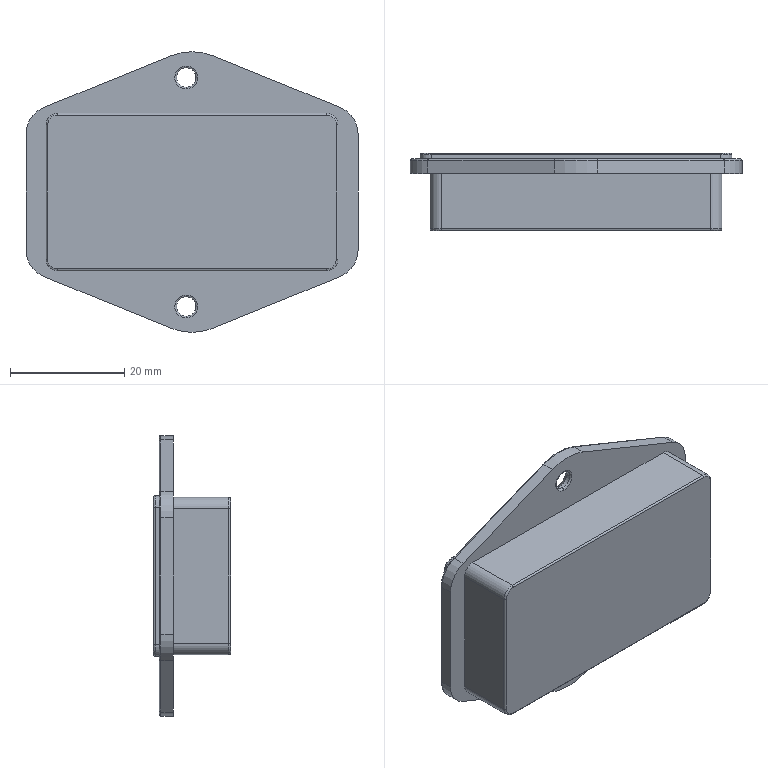Part | SolidWorks | features BaseBody 1 | 1 solid | 74 faces | box 58 x 13.5 x 49 mm | volume 21022 mm3 | cylinder 33 | spline 19 | plane 18 | cone 4 | commonest cylinder face diameters 0.6 x14 4 x8 3.4 x4 10 x4 20 x3